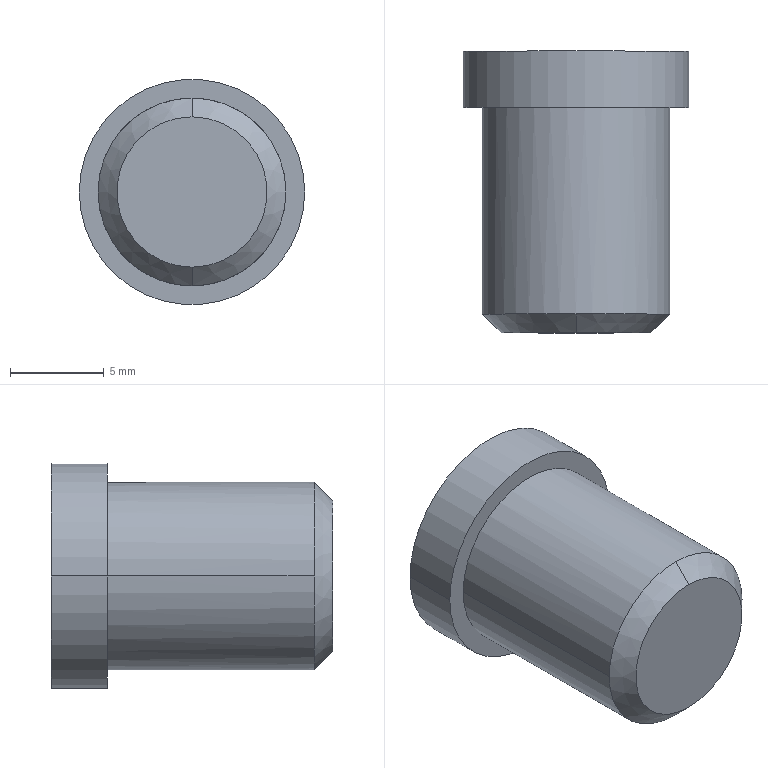Part | SolidWorks | features Chamfer 1, Revolution 1 | 1 solid | 9 faces | box 12 x 15 x 12 mm | volume 1267 mm3 | cylinder 4 | plane 3 | cone 2 | commonest cylinder face diameters 10 x2 12 x2
STEP:
#1=CARTESIAN_POINT('',(104.081,-426.852,-4.));
#2=VERTEX_POINT('',#1);
#3=CARTESIAN_POINT('',(104.081,-426.852,4.));
#4=VERTEX_POINT('',#3);
#5=CARTESIAN_POINT('',(104.081,-426.852,0.));
#6=DIRECTION('',(0.,-1.,0.));
#7=DIRECTION('',(1.,0.,0.));
#8=AXIS2_PLACEMENT_3D('',#5,#6,#7);
#9=CIRCLE('',#8,4.);
#10=EDGE_CURVE('',#2,#4,#9,.T.);
#11=ORIENTED_EDGE('',*,*,#10,.F.);
#12=CARTESIAN_POINT('',(104.081,-425.852,-5.));
#13=VERTEX_POINT('',#12);
#14=CARTESIAN_POINT('',(104.081,-426.852,-4.));
#15=DIRECTION('',(0.,0.7071,-0.7071));
#16=VECTOR('',#15,1000.);
#17=LINE('',#14,#16);
#18=EDGE_CURVE('',#2,#13,#17,.T.);
#19=ORIENTED_EDGE('',*,*,#18,.T.);
#20=CARTESIAN_POINT('',(109.081,-425.852,0.));
#21=VERTEX_POINT('',#20);
#22=CARTESIAN_POINT('',(104.081,-425.852,0.));
#23=DIRECTION('',(0.,1.,0.));
#24=DIRECTION('',(0.,0.,-1.));
#25=AXIS2_PLACEMENT_3D('',#22,#23,#24);
#26=CIRCLE('',#25,5.);
#27=EDGE_CURVE('',#21,#13,#26,.T.);
#28=ORIENTED_EDGE('',*,*,#27,.F.);
#29=CARTESIAN_POINT('',(104.081,-425.852,5.));
#30=VERTEX_POINT('',#29);
#31=CARTESIAN_POINT('',(104.081,-425.852,0.));
#32=DIRECTION('',(0.,1.,0.));
#33=DIRECTION('',(0.,0.,-1.));
#34=AXIS2_PLACEMENT_3D('',#31,#32,#33);
#35=CIRCLE('',#34,5.);
#36=EDGE_CURVE('',#30,#21,#35,.T.);
#37=ORIENTED_EDGE('',*,*,#36,.F.);
#38=CARTESIAN_POINT('',(104.081,-426.852,4.));
#39=DIRECTION('',(0.,0.7071,0.7071));
#40=VECTOR('',#39,1000.);
#41=LINE('',#38,#40);
#42=EDGE_CURVE('',#4,#30,#41,.T.);
#43=ORIENTED_EDGE('',*,*,#42,.F.);
#44=EDGE_LOOP('',(#11,#19,#28,#37,#43));
#45=FACE_OUTER_BOUND('',#44,.T.);
#46=CARTESIAN_POINT('',(104.081,-426.852,0.));
#47=DIRECTION('',(0.,1.,0.));
#48=DIRECTION('',(0.,0.,1.));
#49=AXIS2_PLACEMENT_3D('',#46,#47,#48);
#50=CONICAL_SURFACE('',#49,4.,0.7854);
#51=ADVANCED_FACE('',(#45),#50,.T.);
#52=CARTESIAN_POINT('',(110.081,-411.852,0.));
#53=VERTEX_POINT('',#52);
#54=CARTESIAN_POINT('',(98.081,-411.852,0.));
#55=VERTEX_POINT('',#54);
#56=CARTESIAN_POINT('',(104.081,-411.852,0.));
#57=DIRECTION('',(0.,-1.,0.));
#58=DIRECTION('',(1.,0.,0.));
#59=AXIS2_PLACEMENT_3D('',#56,#57,#58);
#60=CIRCLE('',#59,6.);
#61=EDGE_CURVE('',#53,#55,#60,.T.);
#62=ORIENTED_EDGE('',*,*,#61,.T.);
#63=CARTESIAN_POINT('',(98.081,-414.852,0.));
#64=VERTEX_POINT('',#63);
#65=CARTESIAN_POINT('',(98.081,-427.306,0.));
#66=DIRECTION('',(0.,-1.,0.));
#67=VECTOR('',#66,1000.);
#68=LINE('',#65,#67);
#69=EDGE_CURVE('',#55,#64,#68,.T.);
#70=ORIENTED_EDGE('',*,*,#69,.T.);
#71=CARTESIAN_POINT('',(110.081,-414.852,0.));
#72=VERTEX_POINT('',#71);
#73=CARTESIAN_POINT('',(104.081,-414.852,0.));
#74=DIRECTION('',(0.,-1.,0.));
#75=DIRECTION('',(1.,0.,0.));
#76=AXIS2_PLACEMENT_3D('',#73,#74,#75);
#77=CIRCLE('',#76,6.);
#78=EDGE_CURVE('',#72,#64,#77,.T.);
#79=ORIENTED_EDGE('',*,*,#78,.F.);
#80=CARTESIAN_POINT('',(110.081,-427.306,0.));
#81=DIRECTION('',(0.,-1.,0.));
#82=VECTOR('',#81,1000.);
#83=LINE('',#80,#82);
#84=EDGE_CURVE('',#53,#72,#83,.T.);
#85=ORIENTED_EDGE('',*,*,#84,.F.);
#86=EDGE_LOOP('',(#62,#70,#79,#85));
#87=FACE_OUTER_BOUND('',#86,.T.);
#88=CARTESIAN_POINT('',(104.081,-427.306,0.));
#89=DIRECTION('',(0.,-1.,0.));
#90=DIRECTION('',(1.,0.,0.));
#91=AXIS2_PLACEMENT_3D('',#88,#89,#90);
#92=CYLINDRICAL_SURFACE('',#91,6.);
#93=ADVANCED_FACE('',(#87),#92,.T.);
#94=CARTESIAN_POINT('',(109.081,-414.852,0.));
#95=VERTEX_POINT('',#94);
#96=CARTESIAN_POINT('',(99.081,-414.852,0.));
#97=VERTEX_POINT('',#96);
#98=CARTESIAN_POINT('',(104.081,-414.852,0.));
#99=DIRECTION('',(0.,-1.,0.));
#100=DIRECTION('',(1.,0.,0.));
#101=AXIS2_PLACEMENT_3D('',#98,#99,#100);
#102=CIRCLE('',#101,5.);
#103=EDGE_CURVE('',#95,#97,#102,.T.);
#104=ORIENTED_EDGE('',*,*,#103,.T.);
#105=CARTESIAN_POINT('',(99.081,-425.852,0.));
#106=VERTEX_POINT('',#105);
#107=CARTESIAN_POINT('',(99.081,-427.306,0.));
#108=DIRECTION('',(0.,-1.,0.));
#109=VECTOR('',#108,1000.);
#110=LINE('',#107,#109);
#111=EDGE_CURVE('',#97,#106,#110,.T.);
#112=ORIENTED_EDGE('',*,*,#111,.T.);
#113=CARTESIAN_POINT('',(104.081,-425.852,0.));
#114=DIRECTION('',(0.,1.,0.));
#115=DIRECTION('',(0.,0.,-1.));
#116=AXIS2_PLACEMENT_3D('',#113,#114,#115);
#117=CIRCLE('',#116,5.);
#118=EDGE_CURVE('',#106,#30,#117,.T.);
#119=ORIENTED_EDGE('',*,*,#118,.T.);
#120=ORIENTED_EDGE('',*,*,#36,.T.);
#121=CARTESIAN_POINT('',(109.081,-427.306,0.));
#122=DIRECTION('',(0.,-1.,0.));
#123=VECTOR('',#122,1000.);
#124=LINE('',#121,#123);
#125=EDGE_CURVE('',#95,#21,#124,.T.);
#126=ORIENTED_EDGE('',*,*,#125,.F.);
#127=EDGE_LOOP('',(#104,#112,#119,#120,#126));
#128=FACE_OUTER_BOUND('',#127,.T.);
#129=CARTESIAN_POINT('',(104.081,-427.306,0.));
#130=DIRECTION('',(0.,-1.,0.));
#131=DIRECTION('',(1.,0.,0.));
#132=AXIS2_PLACEMENT_3D('',#129,#130,#131);
#133=CYLINDRICAL_SURFACE('',#132,5.);
#134=ADVANCED_FACE('',(#128),#133,.T.);
#135=ORIENTED_EDGE('',*,*,#61,.F.);
#136=CARTESIAN_POINT('',(104.081,-411.852,0.));
#137=DIRECTION('',(0.,-1.,0.));
#138=DIRECTION('',(1.,0.,0.));
#139=AXIS2_PLACEMENT_3D('',#136,#137,#138);
#140=CIRCLE('',#139,6.);
#141=EDGE_CURVE('',#55,#53,#140,.T.);
#142=ORIENTED_EDGE('',*,*,#141,.F.);
#143=EDGE_LOOP('',(#135,#142));
#144=FACE_OUTER_BOUND('',#143,.T.);
#145=CARTESIAN_POINT('',(110.081,-411.852,0.));
#146=DIRECTION('',(0.,1.,0.));
#147=DIRECTION('',(-1.,0.,0.));
#148=AXIS2_PLACEMENT_3D('',#145,#146,#147);
#149=PLANE('',#148);
#150=ADVANCED_FACE('',(#144),#149,.T.);
#151=CARTESIAN_POINT('',(104.081,-426.852,0.));
#152=DIRECTION('',(0.,-1.,0.));
#153=DIRECTION('',(1.,0.,0.));
#154=AXIS2_PLACEMENT_3D('',#151,#152,#153);
#155=CIRCLE('',#154,4.);
#156=EDGE_CURVE('',#4,#2,#155,.T.);
#157=ORIENTED_EDGE('',*,*,#156,.T.);
#158=ORIENTED_EDGE('',*,*,#10,.T.);
#159=EDGE_LOOP('',(#157,#158));
#160=FACE_OUTER_BOUND('',#159,.T.);
#161=CARTESIAN_POINT('',(104.081,-426.852,0.));
#162=DIRECTION('',(0.,-1.,0.));
#163=DIRECTION('',(1.,0.,0.));
#164=AXIS2_PLACEMENT_3D('',#161,#162,#163);
#165=PLANE('',#164);
#166=ADVANCED_FACE('',(#160),#165,.T.);
#167=ORIENTED_EDGE('',*,*,#111,.F.);
#168=CARTESIAN_POINT('',(104.081,-414.852,0.));
#169=DIRECTION('',(0.,-1.,0.));
#170=DIRECTION('',(1.,0.,0.));
#171=AXIS2_PLACEMENT_3D('',#168,#169,#170);
#172=CIRCLE('',#171,5.);
#173=EDGE_CURVE('',#97,#95,#172,.T.);
#174=ORIENTED_EDGE('',*,*,#173,.T.);
#175=ORIENTED_EDGE('',*,*,#125,.T.);
#176=ORIENTED_EDGE('',*,*,#27,.T.);
#177=CARTESIAN_POINT('',(104.081,-425.852,0.));
#178=DIRECTION('',(0.,1.,0.));
#179=DIRECTION('',(0.,0.,-1.));
#180=AXIS2_PLACEMENT_3D('',#177,#178,#179);
#181=CIRCLE('',#180,5.);
#182=EDGE_CURVE('',#13,#106,#181,.T.);
#183=ORIENTED_EDGE('',*,*,#182,.T.);
#184=EDGE_LOOP('',(#167,#174,#175,#176,#183));
#185=FACE_OUTER_BOUND('',#184,.T.);
#186=CARTESIAN_POINT('',(104.081,-427.306,0.));
#187=DIRECTION('',(0.,-1.,0.));
#188=DIRECTION('',(1.,0.,0.));
#189=AXIS2_PLACEMENT_3D('',#186,#187,#188);
#190=CYLINDRICAL_SURFACE('',#189,5.);
#191=ADVANCED_FACE('',(#185),#190,.T.);
#192=ORIENTED_EDGE('',*,*,#78,.T.);
#193=CARTESIAN_POINT('',(104.081,-414.852,0.));
#194=DIRECTION('',(0.,-1.,0.));
#195=DIRECTION('',(1.,0.,0.));
#196=AXIS2_PLACEMENT_3D('',#193,#194,#195);
#197=CIRCLE('',#196,6.);
#198=EDGE_CURVE('',#64,#72,#197,.T.);
#199=ORIENTED_EDGE('',*,*,#198,.T.);
#200=EDGE_LOOP('',(#192,#199));
#201=FACE_OUTER_BOUND('',#200,.T.);
#202=ORIENTED_EDGE('',*,*,#103,.F.);
#203=ORIENTED_EDGE('',*,*,#173,.F.);
#204=EDGE_LOOP('',(#202,#203));
#205=FACE_BOUND('',#204,.T.);
#206=CARTESIAN_POINT('',(109.081,-414.852,0.));
#207=DIRECTION('',(0.,-1.,0.));
#208=DIRECTION('',(1.,0.,0.));
#209=AXIS2_PLACEMENT_3D('',#206,#207,#208);
#210=PLANE('',#209);
#211=ADVANCED_FACE('',(#201,#205),#210,.T.);
#212=ORIENTED_EDGE('',*,*,#69,.F.);
#213=ORIENTED_EDGE('',*,*,#141,.T.);
#214=ORIENTED_EDGE('',*,*,#84,.T.);
#215=ORIENTED_EDGE('',*,*,#198,.F.);
#216=EDGE_LOOP('',(#212,#213,#214,#215));
#217=FACE_OUTER_BOUND('',#216,.T.);
#218=CARTESIAN_POINT('',(104.081,-427.306,0.));
#219=DIRECTION('',(0.,-1.,0.));
#220=DIRECTION('',(1.,0.,0.));
#221=AXIS2_PLACEMENT_3D('',#218,#219,#220);
#222=CYLINDRICAL_SURFACE('',#221,6.);
#223=ADVANCED_FACE('',(#217),#222,.T.);
#224=ORIENTED_EDGE('',*,*,#18,.F.);
#225=ORIENTED_EDGE('',*,*,#156,.F.);
#226=ORIENTED_EDGE('',*,*,#42,.T.);
#227=ORIENTED_EDGE('',*,*,#118,.F.);
#228=ORIENTED_EDGE('',*,*,#182,.F.);
#229=EDGE_LOOP('',(#224,#225,#226,#227,#228));
#230=FACE_OUTER_BOUND('',#229,.T.);
#231=CARTESIAN_POINT('',(104.081,-426.852,0.));
#232=DIRECTION('',(0.,1.,0.));
#233=DIRECTION('',(0.,0.,1.));
#234=AXIS2_PLACEMENT_3D('',#231,#232,#233);
#235=CONICAL_SURFACE('',#234,4.,0.7854);
#236=ADVANCED_FACE('',(#230),#235,.T.);
#237=CLOSED_SHELL('',(#51,#93,#134,#150,#166,#191,#211,#223,#236));
#238=MANIFOLD_SOLID_BREP('',#237);
#239=CARTESIAN_POINT('',(0.,0.,0.));
#240=DIRECTION('',(0.,0.,1.));
#241=DIRECTION('',(1.,0.,0.));
#242=AXIS2_PLACEMENT_3D('',#239,#240,#241);
#243=(LENGTH_UNIT()NAMED_UNIT(*)SI_UNIT(.MILLI.,.METRE.));
#244=UNCERTAINTY_MEASURE_WITH_UNIT(LENGTH_MEASURE(0.00001),#243,'','');
#245=(NAMED_UNIT(*)PLANE_ANGLE_UNIT()SI_UNIT($,.RADIAN.));
#246=(NAMED_UNIT(*)SI_UNIT($,.STERADIAN.)SOLID_ANGLE_UNIT());
#247=(GEOMETRIC_REPRESENTATION_CONTEXT(3)GLOBAL_UNCERTAINTY_ASSIGNED_CONTEXT((#244))GLOBAL_UNIT_ASSIGNED_CONTEXT((#243,#245,#246))REPRESENTATION_CONTEXT('',''));
#248=ADVANCED_BREP_SHAPE_REPRESENTATION('',(#238,#242),#247);